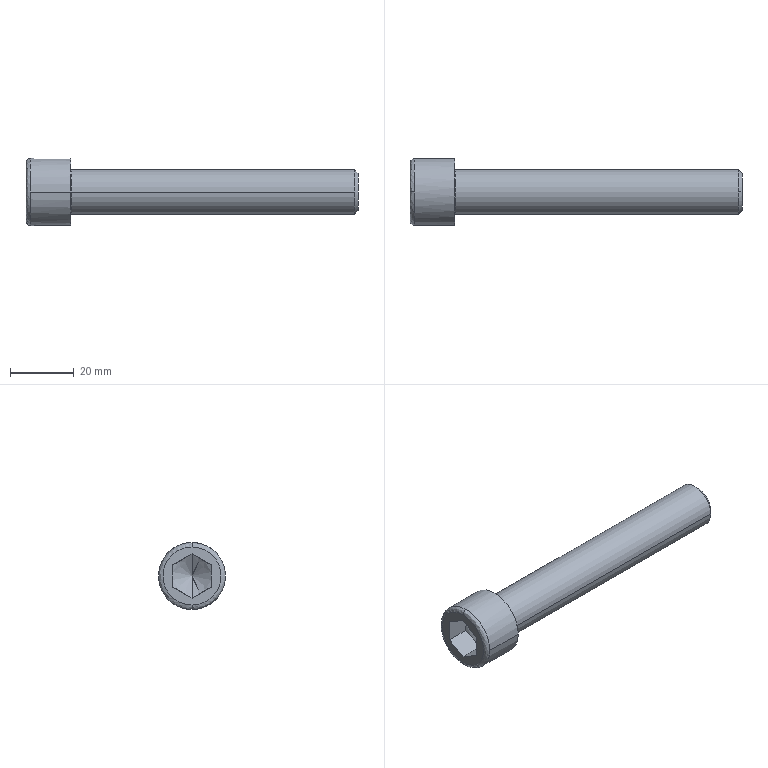Part | STEP file | DIN 912 - replaced by DIN EN ISO 4762 M14 x 90 | 1 solid | 21 faces | box 104 x 21 x 21 mm | volume 17577 mm3 | plane 9 | spline 4 | cylinder 4 | cone 4 | commonest cylinder face diameters 14 x2 21 x2